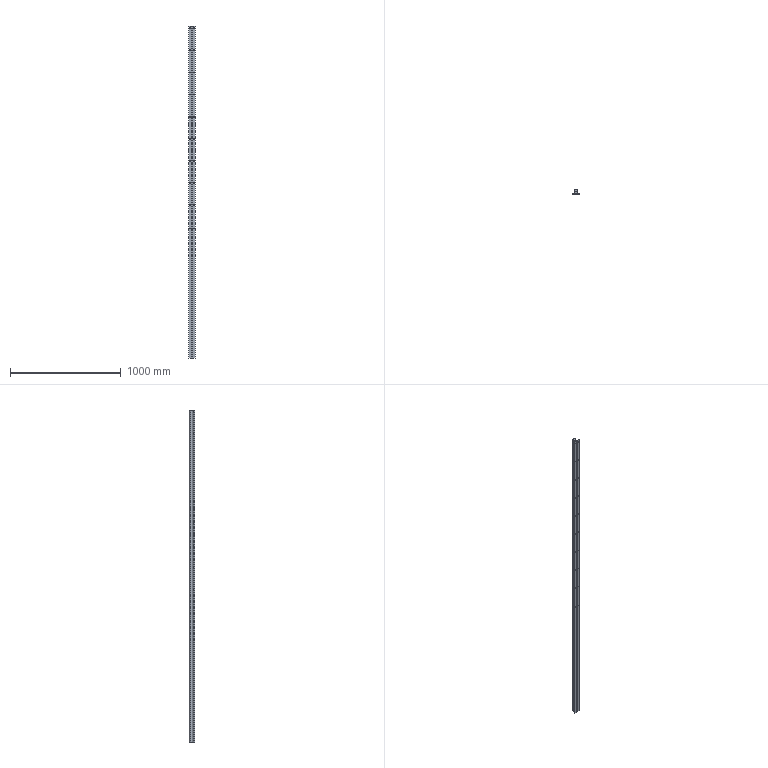Part | SolidWorks | features Chamfer 1, Extrusion 1, ICE 1, MoveFace 1 | 1 solid | 58 faces | box 55 x 45.5 x 3000 mm | volume 2842353 mm3 | cylinder 43 | plane 15 | commonest cylinder face diameters 6.6 x40 25 x3